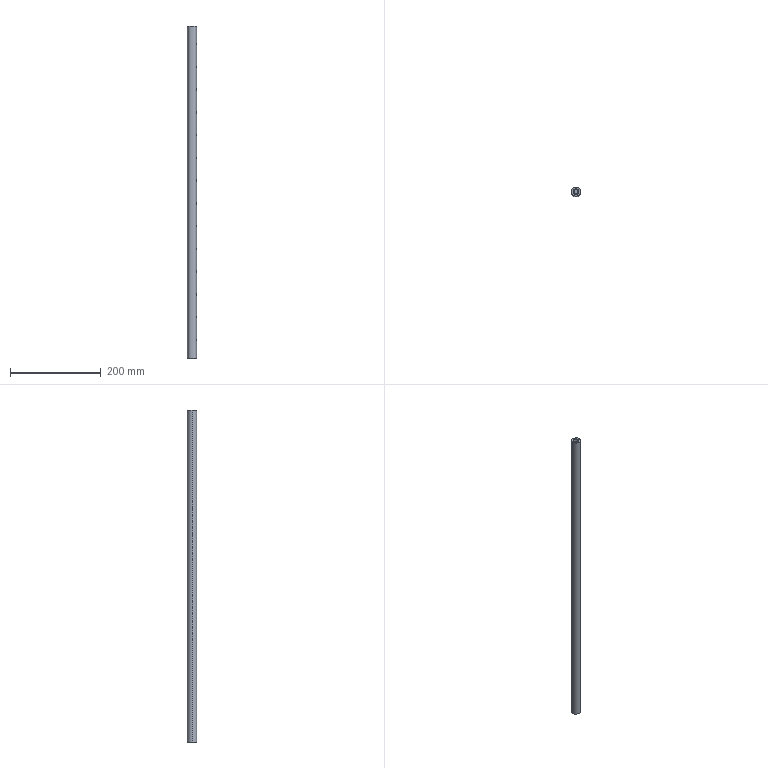Part | STEP file | 2012-06-08-09 | 3 solids | 47 faces | box 20 x 20 x 730 mm | volume 137949 mm3 | cylinder 38 | plane 7 | cone 2 | commonest cylinder face diameters 4.2 x28 12.68 x4 8.433 x2 12.7 x2 20 x2